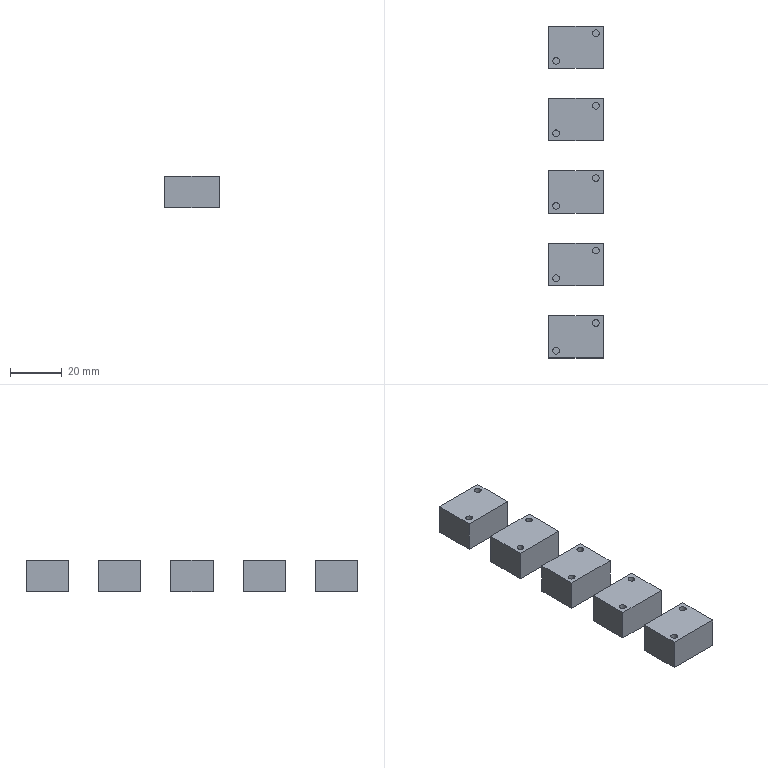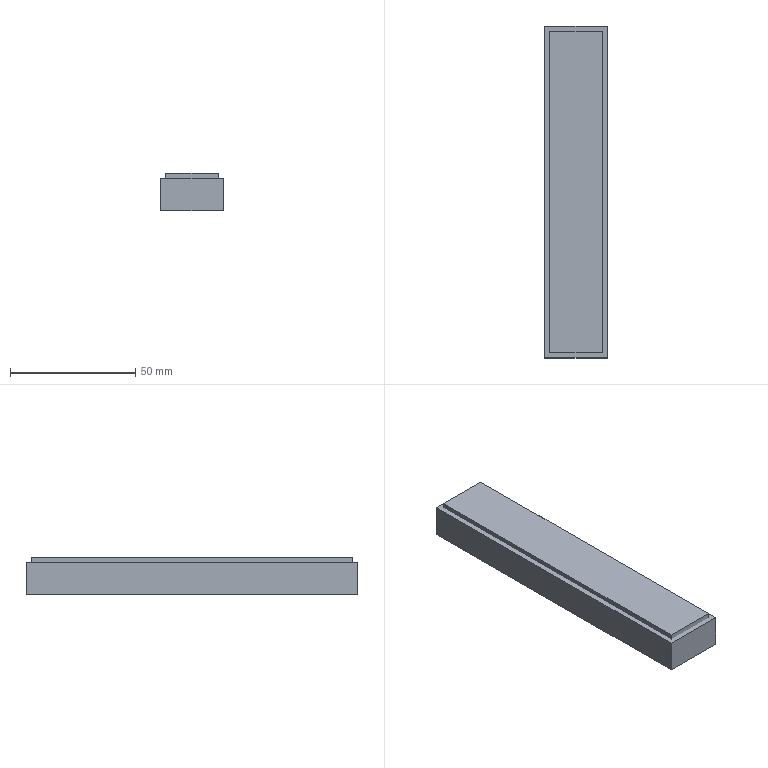CAM job | NX | 3-axis milling, drilling | part box 21 x 128.262 x 12 mm | stock box 25 x 132.262 x 15 mm
Tools:
number,name,description,diameter,corner_radius,flute_length,length,flutes
1,D63,Milling Tool-5 Parameters,63.0,0.0,50.0,75.0,2
7,D6A45,Milling Tool-5 Parameters,6.0,0.0,50.0,75.0,2
12,2.6ZT,Drilling Tool,2.6,0.0,35.0,50.0,2
10,D10,Milling Tool-5 Parameters,10.0,0.0,50.0,75.0,2
Operations:
program,operation,operation_type,tool,method,geometry_group,spindle_rpm,surface_speed,feed_per_tooth,feed_cut,feed_plunge,cut_length_mm,path_length_mm,cut_time_min,machine_time_min
1,FLOOR_WALL,VolumeBased25DMillingOperation,D63,METHOD,A,6500.0,1286.0,0.0962,1250.0,100.0,207.262,261.262,0.1658,0.1712
1,DRILLING,Operation,D6A45,METHOD,A,5000.0,94.0,0.025,250.0,0.0,44.0,363.379,0.176,0.2079
1,DRILLING_COPY,Operation,2.6ZT,METHOD,A,2000.0,16.0,0.03,120.0,0.0,117.811,511.001,0.9818,1.021
1,ZLEVEL_PROFILE,ZLevelMilling,D10,METHOD,A,9500.0,298.0,0.1316,2500.0,1000.0,6927.211,7377.716,2.914,2.959
1,ZLEVEL_PROFILE_COPY,ZLevelMilling,D10,METHOD,A,9500.0,298.0,0.0632,1200.0,1000.0,571.397,1331.065,0.4795,0.5555
1,PLANAR_MILL,PlanarMilling,D6A45,METHOD,A,9500.0,179.0,0.0658,1250.0,100.0,484.122,1594.665,0.3873,0.4984
2,FLOOR_WALL_COPY,VolumeBased25DMillingOperation,D63,METHOD,B,6500.0,1286.0,0.0962,1250.0,100.0,609.787,1160.313,0.4878,0.5429
2,PLANAR_MILL_COPY,PlanarMilling,D6A45,METHOD,B,9500.0,179.0,0.0658,1250.0,100.0,424.626,831.793,0.3397,0.3804